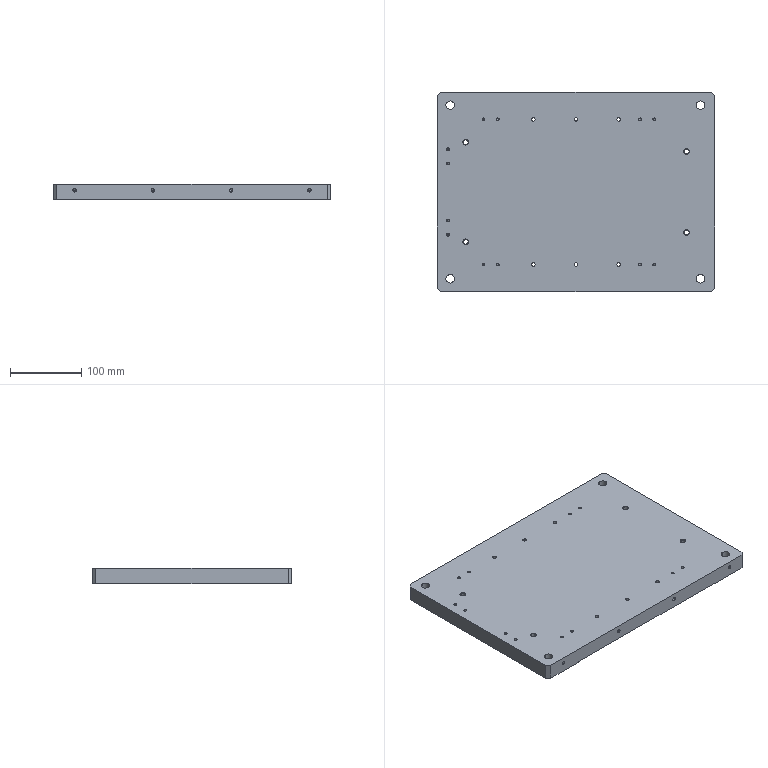NC program | NX | posted with a generic post | part box 390 x 280 x 22 mm
Lines 1876 to 1943 of 1943:
(PLANAR_MILL , TOOL : D6A45)
N3720 T07 M6
N3722 G54
N3724 G17 G0 G90 X-181.6 Y-121.134 S9500 M3
N3726 G43 Z30. H7
N3728 Z2.
N3730 G94 G1 Z-1. F500.
N3732 G3 X-182.1 Y-122. R1.
N3734 X-177. Y-127.1 R5.1 F1250.
N3736 X-182.1 Y-122. R-5.1
N3738 X-181.6 Y-122.866 R1.
N3740 G1 Z2.
N3742 G0 Z30.
N3744 Y122.866
N3746 Z2.
N3748 G1 Z-1. F500.
N3750 G3 X-182.1 Y122. R1.
N3752 X-177. Y116.9 R5.1 F1250.
N3754 X-182.1 Y122. R-5.1
N3756 X-181.6 Y121.134 R1.
N3758 G1 Z2.
N3760 G0 Z30.
N3762 X-0.866 Y141.4
N3764 Z2.
N3766 G1 Z-1. F500.
N3768 G3 X0. Y140.9 R1.
N3770 G1 X190. F1250.
N3772 G2 X190.636 Y140.636 R0.9
N3774 G1 X195.636 Y135.636
N3776 G2 X195.9 Y135. R0.9
N3778 G1 Y-135.
N3780 G2 X195.636 Y-135.636 R0.9
N3782 G1 X190.636 Y-140.636
N3784 G2 X190. Y-140.9 R0.9
N3786 G1 X-190.
N3788 G2 X-190.636 Y-140.636 R0.9
N3790 G1 X-195.636 Y-135.636
N3792 G2 X-195.9 Y-135. R0.9
N3794 G1 Y135.
N3796 G2 X-195.636 Y135.636 R0.9
N3798 G1 X-190.636 Y140.636
N3800 G2 X-190. Y140.9 R0.9
N3802 G1 X0.
N3804 G3 X0.866 Y141.4 R1.
N3806 G1 Z2.
N3808 G0 Z30.
N3810 X175.866 Y126.6
N3812 Z2.
N3814 G1 Z-1. F500.
N3816 G3 X175. Y127.1 R1.
N3818 X169.9 Y122. R5.1 F1250.
N3820 X175. Y127.1 R-5.1
N3822 X174.134 Y126.6 R1.
N3824 G1 Z2.
N3826 G0 Z30.
N3828 Y-126.6
N3830 Z2.
N3832 G1 Z-1. F500.
N3834 G3 X175. Y-127.1 R1.
N3836 X180.1 Y-122. R5.1 F1250.
N3838 X175. Y-127.1 R-5.1
N3840 X175.866 Y-126.6 R1.
N3842 G1 Z2.
N3844 G0 Z30.
N3846 M5
N3848 M2